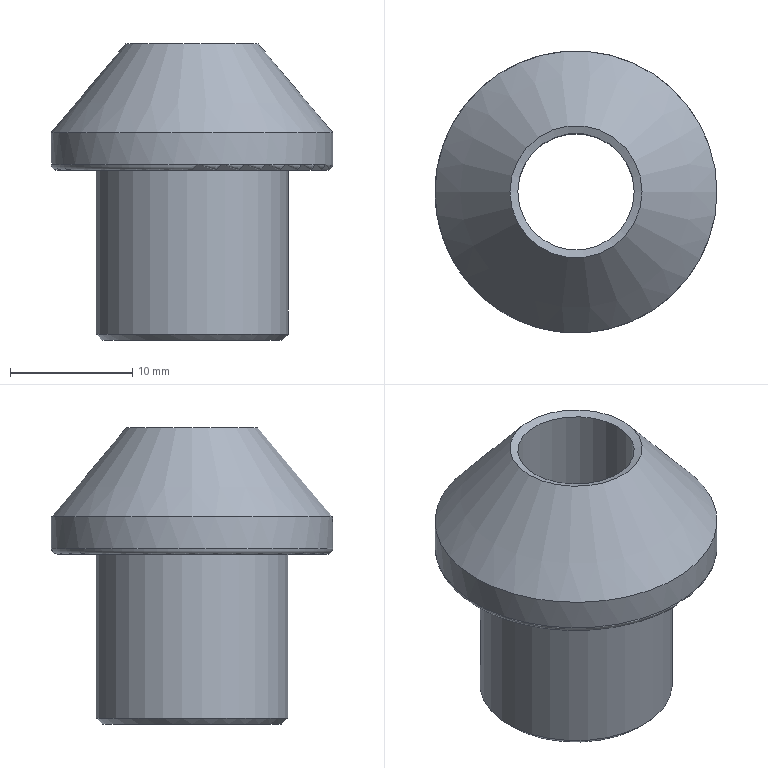Part | NX | features MG0314 tapered end 2 | 1 solid | 12 faces | box 23.05 x 23.05 x 24.234 mm | volume 3562 mm3 | cylinder 4 | cone 3 | plane 3 | torus 2 | commonest cylinder face diameters 9.525 x1 12.446 x1 15.7 x1 23.05 x1
STEP:
#1=CARTESIAN_POINT('',(7.85,0.,-24.5));
#2=VERTEX_POINT('',#1);
#3=CARTESIAN_POINT('',(0.,0.,-24.5));
#4=DIRECTION('',(0.,0.,1.));
#5=DIRECTION('',(1.,0.,0.));
#6=AXIS2_PLACEMENT_3D('',#3,#4,#5);
#7=CIRCLE('',#6,7.85);
#8=EDGE_CURVE('',#2,#2,#7,.T.);
#9=ORIENTED_EDGE('',*,*,#8,.T.);
#10=EDGE_LOOP('',(#9));
#11=FACE_BOUND('',#10,.T.);
#12=CARTESIAN_POINT('',(7.85,0.,-11.112));
#13=VERTEX_POINT('',#12);
#14=CARTESIAN_POINT('',(0.,0.,-11.112));
#15=DIRECTION('',(0.,0.,1.));
#16=DIRECTION('',(1.,0.,0.));
#17=AXIS2_PLACEMENT_3D('',#14,#15,#16);
#18=CIRCLE('',#17,7.85);
#19=EDGE_CURVE('',#13,#13,#18,.T.);
#20=ORIENTED_EDGE('',*,*,#19,.F.);
#21=EDGE_LOOP('',(#20));
#22=FACE_BOUND('',#21,.T.);
#23=CARTESIAN_POINT('',(0.,0.,0.));
#24=DIRECTION('',(0.,0.,1.));
#25=DIRECTION('',(-0.1057,-0.9944,0.));
#26=AXIS2_PLACEMENT_3D('',#23,#24,#25);
#27=CYLINDRICAL_SURFACE('',#26,7.85);
#28=ADVANCED_FACE('',(#11,#22),#27,.T.);
#29=CARTESIAN_POINT('',(-0.6579,-6.188,-18.275));
#30=VERTEX_POINT('',#29);
#31=CARTESIAN_POINT('',(0.,0.,-18.275));
#32=DIRECTION('',(0.,0.,1.));
#33=DIRECTION('',(-0.1057,-0.9944,0.));
#34=AXIS2_PLACEMENT_3D('',#31,#32,#33);
#35=CIRCLE('',#34,6.223);
#36=EDGE_CURVE('',#30,#30,#35,.T.);
#37=ORIENTED_EDGE('',*,*,#36,.T.);
#38=EDGE_LOOP('',(#37));
#39=FACE_BOUND('',#38,.T.);
#40=CARTESIAN_POINT('',(-0.6579,-6.188,-25.));
#41=VERTEX_POINT('',#40);
#42=CARTESIAN_POINT('',(0.,0.,-25.));
#43=DIRECTION('',(0.,0.,1.));
#44=DIRECTION('',(-0.1057,-0.9944,0.));
#45=AXIS2_PLACEMENT_3D('',#42,#43,#44);
#46=CIRCLE('',#45,6.223);
#47=EDGE_CURVE('',#41,#41,#46,.T.);
#48=ORIENTED_EDGE('',*,*,#47,.F.);
#49=EDGE_LOOP('',(#48));
#50=FACE_BOUND('',#49,.T.);
#51=CARTESIAN_POINT('',(0.,0.,0.));
#52=DIRECTION('',(0.,0.,1.));
#53=DIRECTION('',(-0.1057,-0.9944,0.));
#54=AXIS2_PLACEMENT_3D('',#51,#52,#53);
#55=CYLINDRICAL_SURFACE('',#54,6.223);
#56=ADVANCED_FACE('',(#39,#50),#55,.F.);
#57=CARTESIAN_POINT('',(5.405,0.,-0.766));
#58=VERTEX_POINT('',#57);
#59=CARTESIAN_POINT('',(0.,0.,-0.766));
#60=DIRECTION('',(0.,0.,1.));
#61=DIRECTION('',(1.,0.,0.));
#62=AXIS2_PLACEMENT_3D('',#59,#60,#61);
#63=CIRCLE('',#62,5.405);
#64=EDGE_CURVE('',#58,#58,#63,.F.);
#65=ORIENTED_EDGE('',*,*,#64,.T.);
#66=EDGE_LOOP('',(#65));
#67=FACE_BOUND('',#66,.T.);
#68=CARTESIAN_POINT('',(-11.525,0.,-8.059));
#69=VERTEX_POINT('',#68);
#70=CARTESIAN_POINT('',(0.,0.,-8.059));
#71=DIRECTION('',(0.,0.,-1.));
#72=DIRECTION('',(-1.,0.,0.));
#73=AXIS2_PLACEMENT_3D('',#70,#71,#72);
#74=CIRCLE('',#73,11.525);
#75=EDGE_CURVE('',#69,#69,#74,.F.);
#76=ORIENTED_EDGE('',*,*,#75,.T.);
#77=EDGE_LOOP('',(#76));
#78=FACE_BOUND('',#77,.T.);
#79=CARTESIAN_POINT('',(0.,0.,0.));
#80=DIRECTION('',(0.,0.,-1.));
#81=DIRECTION('',(1.,0.,0.));
#82=AXIS2_PLACEMENT_3D('',#79,#80,#81);
#83=CONICAL_SURFACE('',#82,4.762,0.6981);
#84=ADVANCED_FACE('',(#67,#78),#83,.T.);
#85=CARTESIAN_POINT('',(11.525,0.,-10.612));
#86=VERTEX_POINT('',#85);
#87=CARTESIAN_POINT('',(0.,0.,-10.612));
#88=DIRECTION('',(0.,0.,1.));
#89=DIRECTION('',(1.,0.,0.));
#90=AXIS2_PLACEMENT_3D('',#87,#88,#89);
#91=CIRCLE('',#90,11.525);
#92=EDGE_CURVE('',#86,#86,#91,.T.);
#93=ORIENTED_EDGE('',*,*,#92,.T.);
#94=EDGE_LOOP('',(#93));
#95=FACE_BOUND('',#94,.T.);
#96=ORIENTED_EDGE('',*,*,#75,.F.);
#97=EDGE_LOOP('',(#96));
#98=FACE_BOUND('',#97,.T.);
#99=CARTESIAN_POINT('',(0.,0.,0.));
#100=DIRECTION('',(0.,0.,1.));
#101=DIRECTION('',(-0.1057,-0.9944,0.));
#102=AXIS2_PLACEMENT_3D('',#99,#100,#101);
#103=CYLINDRICAL_SURFACE('',#102,11.525);
#104=ADVANCED_FACE('',(#95,#98),#103,.T.);
#105=CARTESIAN_POINT('',(11.025,0.,-11.112));
#106=VERTEX_POINT('',#105);
#107=CARTESIAN_POINT('',(0.,0.,-11.112));
#108=DIRECTION('',(0.,0.,1.));
#109=DIRECTION('',(1.,0.,0.));
#110=AXIS2_PLACEMENT_3D('',#107,#108,#109);
#111=CIRCLE('',#110,11.025);
#112=EDGE_CURVE('',#106,#106,#111,.F.);
#113=ORIENTED_EDGE('',*,*,#112,.T.);
#114=EDGE_LOOP('',(#113));
#115=FACE_BOUND('',#114,.T.);
#116=ORIENTED_EDGE('',*,*,#19,.T.);
#117=EDGE_LOOP('',(#116));
#118=FACE_BOUND('',#117,.T.);
#119=CARTESIAN_POINT('',(7.855,-0.8351,-11.112));
#120=DIRECTION('',(0.,0.,1.));
#121=DIRECTION('',(-0.1057,-0.9944,0.));
#122=AXIS2_PLACEMENT_3D('',#119,#120,#121);
#123=PLANE('',#122);
#124=ADVANCED_FACE('',(#115,#118),#123,.F.);
#125=CARTESIAN_POINT('',(7.35,0.,-25.));
#126=VERTEX_POINT('',#125);
#127=CARTESIAN_POINT('',(0.,0.,-25.));
#128=DIRECTION('',(0.,0.,1.));
#129=DIRECTION('',(1.,0.,0.));
#130=AXIS2_PLACEMENT_3D('',#127,#128,#129);
#131=CIRCLE('',#130,7.35);
#132=EDGE_CURVE('',#126,#126,#131,.F.);
#133=ORIENTED_EDGE('',*,*,#132,.T.);
#134=EDGE_LOOP('',(#133));
#135=FACE_BOUND('',#134,.T.);
#136=ORIENTED_EDGE('',*,*,#47,.T.);
#137=EDGE_LOOP('',(#136));
#138=FACE_BOUND('',#137,.T.);
#139=CARTESIAN_POINT('',(6.188,-0.6579,-25.));
#140=DIRECTION('',(0.,0.,1.));
#141=DIRECTION('',(-0.1057,-0.9944,0.));
#142=AXIS2_PLACEMENT_3D('',#139,#140,#141);
#143=PLANE('',#142);
#144=ADVANCED_FACE('',(#135,#138),#143,.F.);
#145=CARTESIAN_POINT('',(4.762,0.,-17.462));
#146=VERTEX_POINT('',#145);
#147=CARTESIAN_POINT('',(0.,0.,-17.462));
#148=DIRECTION('',(0.,0.,1.));
#149=DIRECTION('',(1.,0.,0.));
#150=AXIS2_PLACEMENT_3D('',#147,#148,#149);
#151=CIRCLE('',#150,4.763);
#152=EDGE_CURVE('',#146,#146,#151,.T.);
#153=ORIENTED_EDGE('',*,*,#152,.T.);
#154=EDGE_LOOP('',(#153));
#155=FACE_BOUND('',#154,.T.);
#156=CARTESIAN_POINT('',(-0.572,-5.38,-17.462));
#157=VERTEX_POINT('',#156);
#158=CARTESIAN_POINT('',(0.,0.,-17.462));
#159=DIRECTION('',(0.,0.,1.));
#160=DIRECTION('',(-0.1057,-0.9944,0.));
#161=AXIS2_PLACEMENT_3D('',#158,#159,#160);
#162=CIRCLE('',#161,5.41);
#163=EDGE_CURVE('',#157,#157,#162,.F.);
#164=ORIENTED_EDGE('',*,*,#163,.T.);
#165=EDGE_LOOP('',(#164));
#166=FACE_BOUND('',#165,.T.);
#167=CARTESIAN_POINT('',(6.188,-0.6579,-17.462));
#168=DIRECTION('',(0.,0.,1.));
#169=DIRECTION('',(-0.1057,-0.9944,0.));
#170=AXIS2_PLACEMENT_3D('',#167,#168,#169);
#171=PLANE('',#170);
#172=ADVANCED_FACE('',(#155,#166),#171,.F.);
#173=ORIENTED_EDGE('',*,*,#163,.F.);
#174=EDGE_LOOP('',(#173));
#175=FACE_BOUND('',#174,.T.);
#176=ORIENTED_EDGE('',*,*,#36,.F.);
#177=EDGE_LOOP('',(#176));
#178=FACE_BOUND('',#177,.T.);
#179=CARTESIAN_POINT('',(0.,0.,-18.275));
#180=DIRECTION('',(0.,0.,1.));
#181=DIRECTION('',(-0.1057,-0.9944,0.));
#182=AXIS2_PLACEMENT_3D('',#179,#180,#181);
#183=TOROIDAL_SURFACE('',#182,5.41,0.8128);
#184=ADVANCED_FACE('',(#175,#178),#183,.F.);
#185=ORIENTED_EDGE('',*,*,#112,.F.);
#186=EDGE_LOOP('',(#185));
#187=FACE_BOUND('',#186,.T.);
#188=ORIENTED_EDGE('',*,*,#92,.F.);
#189=EDGE_LOOP('',(#188));
#190=FACE_BOUND('',#189,.T.);
#191=CARTESIAN_POINT('',(0.,0.,-10.612));
#192=DIRECTION('',(0.,0.,1.));
#193=DIRECTION('',(1.,0.,0.));
#194=AXIS2_PLACEMENT_3D('',#191,#192,#193);
#195=TOROIDAL_SURFACE('',#194,11.025,0.5);
#196=ADVANCED_FACE('',(#187,#190),#195,.T.);
#197=ORIENTED_EDGE('',*,*,#132,.F.);
#198=EDGE_LOOP('',(#197));
#199=FACE_BOUND('',#198,.T.);
#200=ORIENTED_EDGE('',*,*,#8,.F.);
#201=EDGE_LOOP('',(#200));
#202=FACE_BOUND('',#201,.T.);
#203=CARTESIAN_POINT('',(0.,0.,-24.5));
#204=DIRECTION('',(0.,0.,1.));
#205=DIRECTION('',(1.,0.,0.));
#206=AXIS2_PLACEMENT_3D('',#203,#204,#205);
#207=CONICAL_SURFACE('',#206,7.85,0.7854);
#208=ADVANCED_FACE('',(#199,#202),#207,.T.);
#209=CARTESIAN_POINT('',(-4.763,0.,-1.));
#210=VERTEX_POINT('',#209);
#211=CARTESIAN_POINT('',(0.,0.,-1.));
#212=DIRECTION('',(0.,0.,-1.));
#213=DIRECTION('',(-1.,0.,0.));
#214=AXIS2_PLACEMENT_3D('',#211,#212,#213);
#215=CIRCLE('',#214,4.763);
#216=EDGE_CURVE('',#210,#210,#215,.F.);
#217=ORIENTED_EDGE('',*,*,#216,.T.);
#218=EDGE_LOOP('',(#217));
#219=FACE_BOUND('',#218,.T.);
#220=ORIENTED_EDGE('',*,*,#152,.F.);
#221=EDGE_LOOP('',(#220));
#222=FACE_BOUND('',#221,.T.);
#223=CARTESIAN_POINT('',(0.,0.,-0.5292));
#224=DIRECTION('',(0.,0.,-1.));
#225=DIRECTION('',(-1.,0.,0.));
#226=AXIS2_PLACEMENT_3D('',#223,#224,#225);
#227=CYLINDRICAL_SURFACE('',#226,4.763);
#228=ADVANCED_FACE('',(#219,#222),#227,.F.);
#229=ORIENTED_EDGE('',*,*,#216,.F.);
#230=EDGE_LOOP('',(#229));
#231=FACE_BOUND('',#230,.T.);
#232=ORIENTED_EDGE('',*,*,#64,.F.);
#233=EDGE_LOOP('',(#232));
#234=FACE_BOUND('',#233,.T.);
#235=CARTESIAN_POINT('',(0.,0.,-0.766));
#236=DIRECTION('',(0.,0.,1.));
#237=DIRECTION('',(1.,0.,0.));
#238=AXIS2_PLACEMENT_3D('',#235,#236,#237);
#239=CONICAL_SURFACE('',#238,5.405,1.222);
#240=ADVANCED_FACE('',(#231,#234),#239,.F.);
#241=CLOSED_SHELL('',(#28,#56,#84,#104,#124,#144,#172,#184,#196,#208,#228,#240));
#242=MANIFOLD_SOLID_BREP('',#241);
#243=(LENGTH_UNIT()NAMED_UNIT(*)SI_UNIT(.MILLI.,.METRE.));
#244=UNCERTAINTY_MEASURE_WITH_UNIT(LENGTH_MEASURE(0.00001),#243,'','');
#245=(NAMED_UNIT(*)PLANE_ANGLE_UNIT()SI_UNIT($,.RADIAN.));
#246=(NAMED_UNIT(*)SI_UNIT($,.STERADIAN.)SOLID_ANGLE_UNIT());
#247=(GEOMETRIC_REPRESENTATION_CONTEXT(3)GLOBAL_UNCERTAINTY_ASSIGNED_CONTEXT((#244))GLOBAL_UNIT_ASSIGNED_CONTEXT((#243,#245,#246))REPRESENTATION_CONTEXT('',''));
#248=ADVANCED_BREP_SHAPE_REPRESENTATION('',(#242),#247);